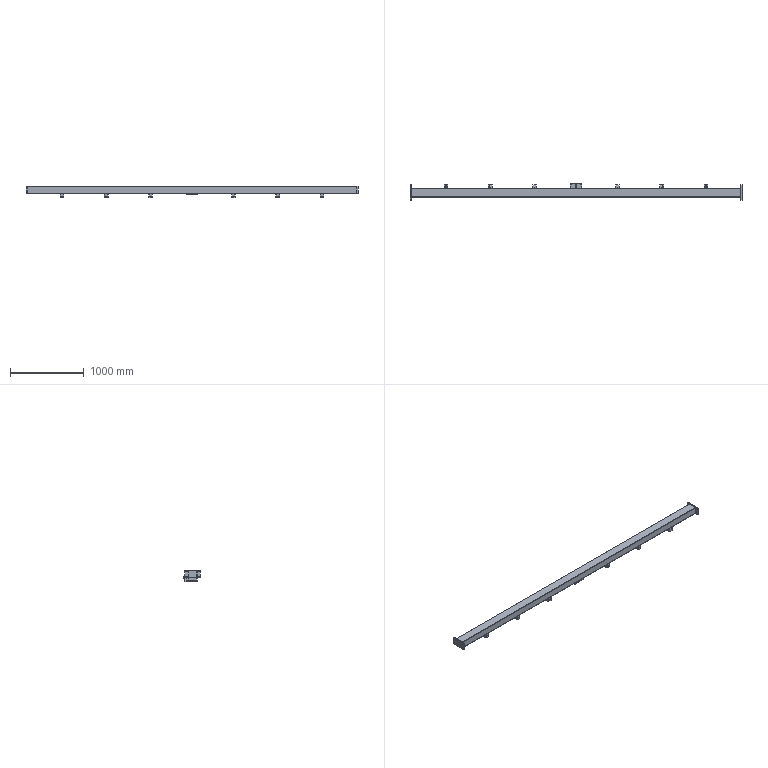Part | SolidWorks | features ICE 5, HoleWzd 3, MirrorSolid 2, WeldMemberFeat 2, LPattern 1, WeldCornerFeat 1, WeldmentFeature 1 | 23 solids | 333 faces | box 4500 x 230 x 153.7 mm | volume 8314769 mm3 | plane 225 | cylinder 108 | commonest cylinder face diameters 5 x24 10 x24 10.2 x24 13.5 x16 8.5 x12 6.4 x4